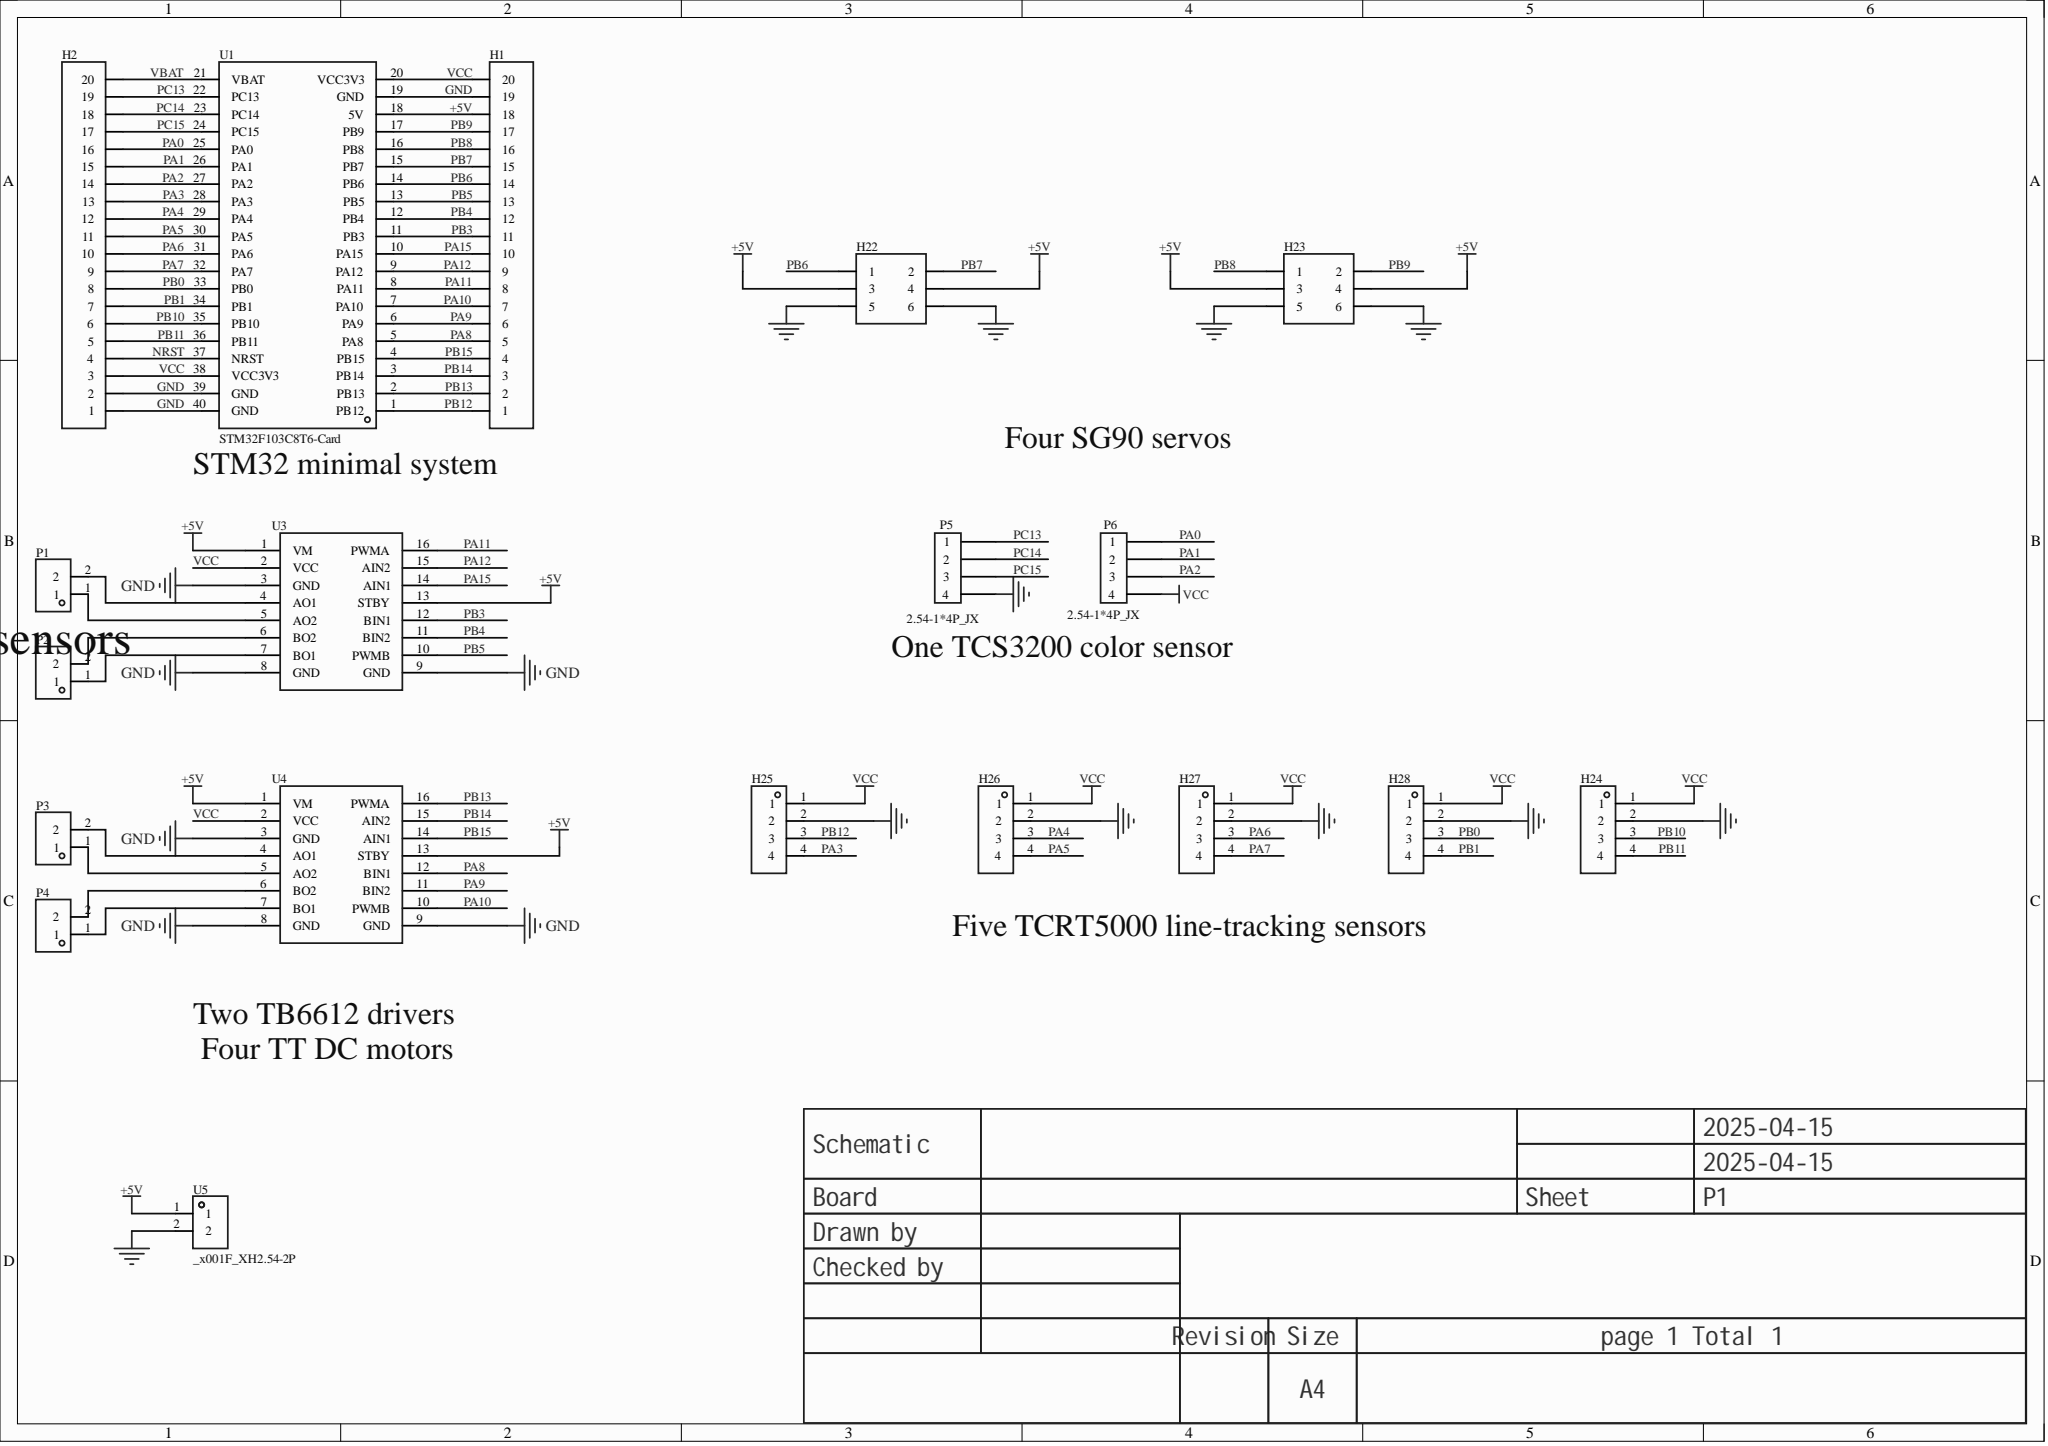Circuit board | Altium Designer | 19 parts | 45 nets
Bill of materials:
Comment,Description,Designator,Footprint,LibRef,Quantity
"","","H1, H2","HDR-TH_20P-P2.54-V-F","HDR-F_2.54_1x20P","2"
"","","H22, H23","HDR-TH_6P-P2.54-V-F-R2-C3-S2.54","HDR-F_2.54_2x3","2"
"","","H24, H25, H26, H27, H28","HDR-TH_4P-P2.54-V-M","HDR-M_2.54_1x4P","5"
"KF301-2P terminal block","","P1, P2, P3, P4","CONN-TH_XY301V-A-5.0-2P","KF301-2P接线端子","4"
"2.54-1*4P_JX","","P5, P6","2.54-1*4P_JX","C2337","2"
"STM32F103C8T6-Card","","U1","CONN-TH_L53.3-W22.9_STM32F103C8T6-CARD","STM32F103C8T6-Card","1"
"","","U3, U4","tb6612","tb6612","2"
"_x001F_XH2.54-2P","","U5","CONN-TH_2P-P2.54-V","_x001F_XH2.54-2P","1"
Netlist (Protel format):
[
H1
HDR-TH_20P-P2.54-V-F




]
[
H2
HDR-TH_20P-P2.54-V-F




]
[
H22
HDR-TH_6P-P2.54-V-F-R2-C3-S2.54




]
[
H23
HDR-TH_6P-P2.54-V-F-R2-C3-S2.54




]
[
H24
HDR-TH_4P-P2.54-V-M




]
[
H25
HDR-TH_4P-P2.54-V-M




]
[
H26
HDR-TH_4P-P2.54-V-M




]
[
H27
HDR-TH_4P-P2.54-V-M




]
[
H28
HDR-TH_4P-P2.54-V-M




]
[
P1
CONN-TH_XY301V-A-5.0-2P
KF301-2P terminal block



]
[
P2
CONN-TH_XY301V-A-5.0-2P
KF301-2P terminal block



]
[
P3
CONN-TH_XY301V-A-5.0-2P
KF301-2P terminal block



]
[
P4
CONN-TH_XY301V-A-5.0-2P
KF301-2P terminal block



]
[
P5
2.54-1*4P_JX
2.54-1*4P_JX



]
[
P6
2.54-1*4P_JX
2.54-1*4P_JX



]
[
U1
CONN-TH_L53.3-W22.9_STM32F103C8T6-CARD
STM32F103C8T6-Card



]
[
U3
tb6612




]
[
U4
tb6612




]
[
U5
CONN-TH_2P-P2.54-V
_x001F_XH2.54-2P



]
(
VCC
H1-20
H2-3
H24-1
H25-1
H26-1
H27-1
H28-1
P6-4
U1-20
U1-38
U3-2
U4-2
)
(
VBAT
H2-20
U1-21
)
(
PC15
H2-17
P5-3
U1-24
)
(
PC14
H2-18
P5-2
U1-23
)
(
PC13
H2-19
P5-1
U1-22
)
(
PB15
H1-4
U1-4
U4-14
)
(
PB14
H1-3
U1-3
U4-15
)
(
PB13
H1-2
U1-2
U4-16
)
(
PB12
H1-1
H25-3
U1-1
)
(
PB11
H2-5
H24-4
U1-36
)
(
PB10
H2-6
H24-3
U1-35
)
(
PB9
H1-17
H23-2
U1-17
)
(
PB8
H1-16
H23-1
U1-16
)
(
PB7
H1-15
H22-2
U1-15
)
(
PB6
H1-14
H22-1
U1-14
)
(
PB5
H1-13
U1-13
U3-10
)
(
PB4
H1-12
U1-12
U3-11
)
(
PB3
H1-11
U1-11
U3-12
)
(
PB1
H2-7
H28-4
U1-34
)
(
PB0
H2-8
H28-3
U1-33
)
(
PA15
H1-10
U1-10
U3-14
)
(
PA12
H1-9
U1-9
U3-15
)
(
PA11
H1-8
U1-8
U3-16
)
(
PA10
H1-7
U1-7
U4-10
)
(
PA9
H1-6
U1-6
U4-11
)
(
PA8
H1-5
U1-5
U4-12
)
(
PA7
H2-9
H27-4
U1-32
)
(
PA6
H2-10
H27-3
U1-31
)
(
PA5
H2-11
H26-4
U1-30
)
(
PA4
H2-12
H26-3
U1-29
)
(
PA3
H2-13
H25-4
U1-28
)
(
PA2
H2-14
P6-3
U1-27
)
(
PA1
H2-15
P6-2
U1-26
)
(
PA0
H2-16
P6-1
U1-25
)
(
NRST
H2-4
U1-37
)
(
NetP4_2
P4-2
U4-6
)
(
NetP4_1
P4-1
U4-7
)
(
NetP3_2
P3-2
U4-4
)
(
NetP3_1
P3-1
U4-5
)
(
NetP2_2
P2-2
U3-6
)
(
NetP2_1
P2-1
U3-7
)
(
NetP1_2
P1-2
U3-4
)
(
NetP1_1
P1-1
U3-5
)
(
GND
H1-19
H2-1
H2-2
H22-5
H22-6
H23-5
H23-6
H24-2
H25-2
H26-2
H27-2
H28-2
P5-4
U1-19
U1-39
U1-40
U3-3
U3-8
U3-9
U4-3
U4-8
U4-9
U5-2
)
(
+5V
H1-18
H22-3
H22-4
H23-3
H23-4
U1-18
U3-1
U3-13
U4-1
U4-13
U5-1
)